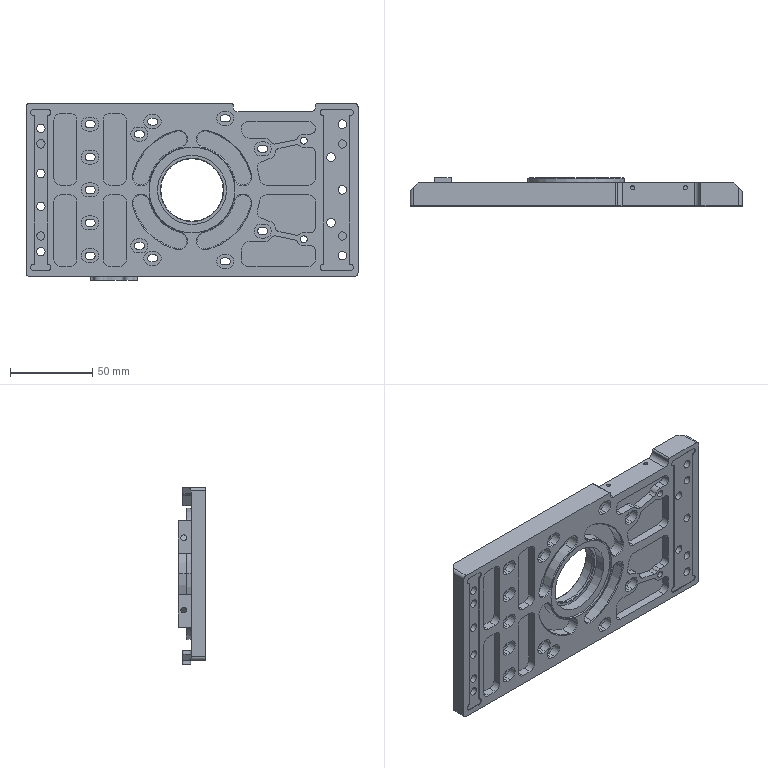NC program | Mastercam | posted with a generic post | part box 202 x 17 x 107.5 mm
Lines 3574 to 4550 of 36425:
(6 FEM |TOOL - 6|DIA. OFF. - 6|LEN. - 6|TOOL DIA. - 6.)
N7212 T6 M6
N7214 G0 G54 G90 X68.194 Y51.5 C0. B0. S6500 M3
N7216 G43 H6 Z100.
N7218 Z1.
N7220 G1 Z-.494 F600.
N7222 Y50.9 F3000.
N7224 G3 X68.494 Y50.6 I.3
N7226 G1 X71.9
N7228 Y51.5
N7230 G2 X72.969 Y54.261 I4.1
N7232 G3 X73.047 Y54.463 I-.222 J.202
N7234 X72.949 Y54.685 I-.3
N7236 G1 X72.506 Y55.089
N7238 X68.194 Y51.5
N7240 Z-.988 F600.
N7242 Y50.9 F3000.
N7244 G3 X68.494 Y50.6 I.3
N7246 G1 X71.9
N7248 Y51.5
N7250 G2 X72.969 Y54.261 I4.1
N7252 G3 X73.047 Y54.463 I-.222 J.202
N7254 X72.949 Y54.685 I-.3
N7256 G1 X72.506 Y55.089
N7258 X68.194 Y51.5
N7260 Z-1.482 F600.
N7262 Y50.9 F3000.
N7264 G3 X68.494 Y50.6 I.3
N7266 G1 X71.9
N7268 Y51.5
N7270 G2 X72.969 Y54.261 I4.1
N7272 G3 X73.047 Y54.463 I-.222 J.202
N7274 X72.949 Y54.685 I-.3
N7276 G1 X72.506 Y55.089
N7278 X68.194 Y51.5
N7280 Z-1.976 F600.
N7282 Y50.9 F3000.
N7284 G3 X68.494 Y50.6 I.3
N7286 G1 X71.9
N7288 Y51.5
N7290 G2 X72.969 Y54.261 I4.1
N7292 G3 X73.047 Y54.463 I-.222 J.202
N7294 X72.949 Y54.685 I-.3
N7296 G1 X72.506 Y55.089
N7298 X68.194 Y51.5
N7300 Z-2.471 F600.
N7302 Y50.9 F3000.
N7304 G3 X68.494 Y50.6 I.3
N7306 G1 X71.9
N7308 Y51.5
N7310 G2 X72.969 Y54.261 I4.1
N7312 G3 X73.047 Y54.463 I-.222 J.202
N7314 X72.949 Y54.685 I-.3
N7316 G1 X72.506 Y55.089
N7318 X68.194 Y51.5
N7320 Z-2.965 F600.
N7322 Y50.9 F3000.
N7324 G3 X68.494 Y50.6 I.3
N7326 G1 X71.9
N7328 Y51.5
N7330 G2 X72.969 Y54.261 I4.1
N7332 G3 X73.047 Y54.463 I-.222 J.202
N7334 X72.949 Y54.685 I-.3
N7336 G1 X72.506 Y55.089
N7338 X68.194 Y51.5
N7340 Z-3.459 F600.
N7342 Y50.9 F3000.
N7344 G3 X68.494 Y50.6 I.3
N7346 G1 X71.9
N7348 Y51.5
N7350 G2 X72.969 Y54.261 I4.1
N7352 G3 X73.047 Y54.463 I-.222 J.202
N7354 X72.949 Y54.685 I-.3
N7356 G1 X72.506 Y55.089
N7358 X68.194 Y51.5
N7360 Z-3.953 F600.
N7362 Y50.9 F3000.
N7364 G3 X68.494 Y50.6 I.3
N7366 G1 X71.9
N7368 Y51.5
N7370 G2 X72.969 Y54.261 I4.1
N7372 G3 X73.047 Y54.463 I-.222 J.202
N7374 X72.949 Y54.685 I-.3
N7376 G1 X72.506 Y55.089
N7378 X68.194 Y51.5
N7380 Z-4.447 F600.
N7382 Y50.9 F3000.
N7384 G3 X68.494 Y50.6 I.3
N7386 G1 X71.9
N7388 Y51.5
N7390 G2 X72.969 Y54.261 I4.1
N7392 G3 X73.047 Y54.463 I-.222 J.202
N7394 X72.949 Y54.685 I-.3
N7396 G1 X72.506 Y55.089
N7398 X68.194 Y51.5
N7400 Z-4.941 F600.
N7402 Y50.9 F3000.
N7404 G3 X68.494 Y50.6 I.3
N7406 G1 X71.9
N7408 Y51.5
N7410 G2 X72.969 Y54.261 I4.1
N7412 G3 X73.047 Y54.463 I-.222 J.202
N7414 X72.949 Y54.685 I-.3
N7416 G1 X72.506 Y55.089
N7418 X68.194 Y51.5
N7420 Z-5.435 F600.
N7422 Y50.9 F3000.
N7424 G3 X68.494 Y50.6 I.3
N7426 G1 X71.9
N7428 Y51.5
N7430 G2 X72.969 Y54.261 I4.1
N7432 G3 X73.047 Y54.463 I-.222 J.202
N7434 X72.949 Y54.685 I-.3
N7436 G1 X72.506 Y55.089
N7438 X68.194 Y51.5
N7440 Z-5.929 F600.
N7442 Y50.9 F3000.
N7444 G3 X68.494 Y50.6 I.3
N7446 G1 X71.9
N7448 Y51.5
N7450 G2 X72.969 Y54.261 I4.1
N7452 G3 X73.047 Y54.463 I-.222 J.202
N7454 X72.949 Y54.685 I-.3
N7456 G1 X72.506 Y55.089
N7458 X68.194 Y51.5
N7460 Z-6.424 F600.
N7462 Y50.9 F3000.
N7464 G3 X68.494 Y50.6 I.3
N7466 G1 X71.9
N7468 Y51.5
N7470 G2 X72.969 Y54.261 I4.1
N7472 G3 X73.047 Y54.463 I-.222 J.202
N7474 X72.949 Y54.685 I-.3
N7476 G1 X72.506 Y55.089
N7478 X68.194 Y51.5
N7480 Z-6.918 F600.
N7482 Y50.9 F3000.
N7484 G3 X68.494 Y50.6 I.3
N7486 G1 X71.9
N7488 Y51.5
N7490 G2 X72.969 Y54.261 I4.1
N7492 G3 X73.047 Y54.463 I-.222 J.202
N7494 X72.949 Y54.685 I-.3
N7496 G1 X72.506 Y55.089
N7498 X68.194 Y51.5
N7500 Z-7.412 F600.
N7502 Y50.9 F3000.
N7504 G3 X68.494 Y50.6 I.3
N7506 G1 X71.9
N7508 Y51.5
N7510 G2 X72.969 Y54.261 I4.1
N7512 G3 X73.047 Y54.463 I-.222 J.202
N7514 X72.949 Y54.685 I-.3
N7516 G1 X72.506 Y55.089
N7518 X68.194 Y51.5
N7520 Z-7.906 F600.
N7522 Y50.9 F3000.
N7524 G3 X68.494 Y50.6 I.3
N7526 G1 X71.9
N7528 Y51.5
N7530 G2 X72.969 Y54.261 I4.1
N7532 G3 X73.047 Y54.463 I-.222 J.202
N7534 X72.949 Y54.685 I-.3
N7536 G1 X72.506 Y55.089
N7538 X68.194 Y51.5
N7540 Z-8.4 F600.
N7542 Y50.9 F3000.
N7544 G3 X68.494 Y50.6 I.3
N7546 G1 X71.9
N7548 Y51.5
N7550 G2 X72.969 Y54.261 I4.1
N7552 G3 X73.047 Y54.463 I-.222 J.202
N7554 X72.949 Y54.685 I-.3
N7556 G1 X72.506 Y55.089
N7558 X68.194 Y51.5
N7560 Z-8.894 F600.
N7562 Y50.9 F3000.
N7564 G3 X68.494 Y50.6 I.3
N7566 G1 X71.9
N7568 Y51.5
N7570 G2 X72.969 Y54.261 I4.1
N7572 G3 X73.047 Y54.463 I-.222 J.202
N7574 X72.949 Y54.685 I-.3
N7576 G1 X72.506 Y55.089
N7578 X68.194 Y51.5
N7580 Z-9.388 F600.
N7582 Y50.9 F3000.
N7584 G3 X68.494 Y50.6 I.3
N7586 G1 X71.9
N7588 Y51.5
N7590 G2 X72.969 Y54.261 I4.1
N7592 G3 X73.047 Y54.463 I-.222 J.202
N7594 X72.949 Y54.685 I-.3
N7596 G1 X72.506 Y55.089
N7598 X68.194 Y51.5
N7600 Z-9.882 F600.
N7602 Y50.9 F3000.
N7604 G3 X68.494 Y50.6 I.3
N7606 G1 X71.9
N7608 Y51.5
N7610 G2 X72.969 Y54.261 I4.1
N7612 G3 X73.047 Y54.463 I-.222 J.202
N7614 X72.949 Y54.685 I-.3
N7616 G1 X72.506 Y55.089
N7618 X68.194 Y51.5
N7620 Z-10.376 F600.
N7622 Y50.9 F3000.
N7624 G3 X68.494 Y50.6 I.3
N7626 G1 X71.9
N7628 Y51.5
N7630 G2 X72.969 Y54.261 I4.1
N7632 G3 X73.047 Y54.463 I-.222 J.202
N7634 X72.949 Y54.685 I-.3
N7636 G1 X72.506 Y55.089
N7638 X68.194 Y51.5
N7640 Z-10.871 F600.
N7642 Y50.9 F3000.
N7644 G3 X68.494 Y50.6 I.3
N7646 G1 X71.9
N7648 Y51.5
N7650 G2 X72.969 Y54.261 I4.1
N7652 G3 X73.047 Y54.463 I-.222 J.202
N7654 X72.949 Y54.685 I-.3
N7656 G1 X72.506 Y55.089
N7658 X68.194 Y51.5
N7660 Z-11.365 F600.
N7662 Y50.9 F3000.
N7664 G3 X68.494 Y50.6 I.3
N7666 G1 X71.9
N7668 Y51.5
N7670 G2 X72.969 Y54.261 I4.1
N7672 G3 X73.047 Y54.463 I-.222 J.202
N7674 X72.949 Y54.685 I-.3
N7676 G1 X72.506 Y55.089
N7678 X68.194 Y51.5
N7680 Z-11.859 F600.
N7682 Y50.9 F3000.
N7684 G3 X68.494 Y50.6 I.3
N7686 G1 X71.9
N7688 Y51.5
N7690 G2 X72.969 Y54.261 I4.1
N7692 G3 X73.047 Y54.463 I-.222 J.202
N7694 X72.949 Y54.685 I-.3
N7696 G1 X72.506 Y55.089
N7698 X68.194 Y51.5
N7700 Z-12.353 F600.
N7702 Y50.9 F3000.
N7704 G3 X68.494 Y50.6 I.3
N7706 G1 X71.9
N7708 Y51.5
N7710 G2 X72.969 Y54.261 I4.1
N7712 G3 X73.047 Y54.463 I-.222 J.202
N7714 X72.949 Y54.685 I-.3
N7716 G1 X72.506 Y55.089
N7718 X68.194 Y51.5
N7720 Z-12.847 F600.
N7722 Y50.9 F3000.
N7724 G3 X68.494 Y50.6 I.3
N7726 G1 X71.9
N7728 Y51.5
N7730 G2 X72.969 Y54.261 I4.1
N7732 G3 X73.047 Y54.463 I-.222 J.202
N7734 X72.949 Y54.685 I-.3
N7736 G1 X72.506 Y55.089
N7738 X68.194 Y51.5
N7740 Z-13.341 F600.
N7742 Y50.9 F3000.
N7744 G3 X68.494 Y50.6 I.3
N7746 G1 X71.9
N7748 Y51.5
N7750 G2 X72.969 Y54.261 I4.1
N7752 G3 X73.047 Y54.463 I-.222 J.202
N7754 X72.949 Y54.685 I-.3
N7756 G1 X72.506 Y55.089
N7758 X68.194 Y51.5
N7760 Z-13.835 F600.
N7762 Y50.9 F3000.
N7764 G3 X68.494 Y50.6 I.3
N7766 G1 X71.9
N7768 Y51.5
N7770 G2 X72.969 Y54.261 I4.1
N7772 G3 X73.047 Y54.463 I-.222 J.202
N7774 X72.949 Y54.685 I-.3
N7776 G1 X72.506 Y55.089
N7778 X68.194 Y51.5
N7780 Z-14.329 F600.
N7782 Y50.9 F3000.
N7784 G3 X68.494 Y50.6 I.3
N7786 G1 X71.9
N7788 Y51.5
N7790 G2 X72.969 Y54.261 I4.1
N7792 G3 X73.047 Y54.463 I-.222 J.202
N7794 X72.949 Y54.685 I-.3
N7796 G1 X72.506 Y55.089
N7798 X68.194 Y51.5
N7800 Z-14.824 F600.
N7802 Y50.9 F3000.
N7804 G3 X68.494 Y50.6 I.3
N7806 G1 X71.9
N7808 Y51.5
N7810 G2 X72.969 Y54.261 I4.1
N7812 G3 X73.047 Y54.463 I-.222 J.202
N7814 X72.949 Y54.685 I-.3
N7816 G1 X72.506 Y55.089
N7818 X68.194 Y51.5
N7820 Z-15.318 F600.
N7822 Y50.9 F3000.
N7824 G3 X68.494 Y50.6 I.3
N7826 G1 X71.9
N7828 Y51.5
N7830 G2 X72.969 Y54.261 I4.1
N7832 G3 X73.047 Y54.463 I-.222 J.202
N7834 X72.949 Y54.685 I-.3
N7836 G1 X72.506 Y55.089
N7838 X68.194 Y51.5
N7840 Z-15.812 F600.
N7842 Y50.9 F3000.
N7844 G3 X68.494 Y50.6 I.3
N7846 G1 X71.9
N7848 Y51.5
N7850 G2 X72.969 Y54.261 I4.1
N7852 G3 X73.047 Y54.463 I-.222 J.202
N7854 X72.949 Y54.685 I-.3
N7856 G1 X72.506 Y55.089
N7858 X68.194 Y51.5
N7860 Z-16.306 F600.
N7862 Y50.9 F3000.
N7864 G3 X68.494 Y50.6 I.3
N7866 G1 X71.9
N7868 Y51.5
N7870 G2 X72.969 Y54.261 I4.1
N7872 G3 X73.047 Y54.463 I-.222 J.202
N7874 X72.949 Y54.685 I-.3
N7876 G1 X72.506 Y55.089
N7878 X68.194 Y51.5
N7880 Z-16.8 F600.
N7882 Y50.9 F3000.
N7884 G3 X68.494 Y50.6 I.3
N7886 G1 X71.9
N7888 Y51.5
N7890 G2 X72.969 Y54.261 I4.1
N7892 G3 X73.047 Y54.463 I-.222 J.202
N7894 X72.949 Y54.685 I-.3
N7896 G1 X72.506 Y55.089
N7898 Z-15.8 F1200.
N7900 G0 Z100.
N7902 X27.48 Y55.103
N7904 Z1.
N7906 G1 Z-.494 F600.
N7908 X27.038 Y54.697 F3000.
N7910 G3 X26.941 Y54.476 I.203 J-.221
N7912 X27.02 Y54.273 I.3
N7914 G2 X28.1 Y51.5 I-3.02 J-2.773
N7916 G1 Y50.6
N7918 X31.52
N7920 G3 X31.82 Y50.9 J.3
N7922 G1 Y51.5
N7924 X27.48 Y55.103
N7926 Z-.988 F600.
N7928 X27.038 Y54.697 F3000.
N7930 G3 X26.941 Y54.476 I.203 J-.221
N7932 X27.02 Y54.273 I.3
N7934 G2 X28.1 Y51.5 I-3.02 J-2.773
N7936 G1 Y50.6
N7938 X31.52
N7940 G3 X31.82 Y50.9 J.3
N7942 G1 Y51.5
N7944 X27.48 Y55.103
N7946 Z-1.482 F600.
N7948 X27.038 Y54.697 F3000.
N7950 G3 X26.941 Y54.476 I.203 J-.221
N7952 X27.02 Y54.273 I.3
N7954 G2 X28.1 Y51.5 I-3.02 J-2.773
N7956 G1 Y50.6
N7958 X31.52
N7960 G3 X31.82 Y50.9 J.3
N7962 G1 Y51.5
N7964 X27.48 Y55.103
N7966 Z-1.976 F600.
N7968 X27.038 Y54.697 F3000.
N7970 G3 X26.941 Y54.476 I.203 J-.221
N7972 X27.02 Y54.273 I.3
N7974 G2 X28.1 Y51.5 I-3.02 J-2.773
N7976 G1 Y50.6
N7978 X31.52
N7980 G3 X31.82 Y50.9 J.3
N7982 G1 Y51.5
N7984 X27.48 Y55.103
N7986 Z-2.471 F600.
N7988 X27.038 Y54.697 F3000.
N7990 G3 X26.941 Y54.476 I.203 J-.221
N7992 X27.02 Y54.273 I.3
N7994 G2 X28.1 Y51.5 I-3.02 J-2.773
N7996 G1 Y50.6
N7998 X31.52
N8000 G3 X31.82 Y50.9 J.3
N8002 G1 Y51.5
N8004 X27.48 Y55.103
N8006 Z-2.965 F600.
N8008 X27.038 Y54.697 F3000.
N8010 G3 X26.941 Y54.476 I.203 J-.221
N8012 X27.02 Y54.273 I.3
N8014 G2 X28.1 Y51.5 I-3.02 J-2.773
N8016 G1 Y50.6
N8018 X31.52
N8020 G3 X31.82 Y50.9 J.3
N8022 G1 Y51.5
N8024 X27.48 Y55.103
N8026 Z-3.459 F600.
N8028 X27.038 Y54.697 F3000.
N8030 G3 X26.941 Y54.476 I.203 J-.221
N8032 X27.02 Y54.273 I.3
N8034 G2 X28.1 Y51.5 I-3.02 J-2.773
N8036 G1 Y50.6
N8038 X31.52
N8040 G3 X31.82 Y50.9 J.3
N8042 G1 Y51.5
N8044 X27.48 Y55.103
N8046 Z-3.953 F600.
N8048 X27.038 Y54.697 F3000.
N8050 G3 X26.941 Y54.476 I.203 J-.221
N8052 X27.02 Y54.273 I.3
N8054 G2 X28.1 Y51.5 I-3.02 J-2.773
N8056 G1 Y50.6
N8058 X31.52
N8060 G3 X31.82 Y50.9 J.3
N8062 G1 Y51.5
N8064 X27.48 Y55.103
N8066 Z-4.447 F600.
N8068 X27.038 Y54.697 F3000.
N8070 G3 X26.941 Y54.476 I.203 J-.221
N8072 X27.02 Y54.273 I.3
N8074 G2 X28.1 Y51.5 I-3.02 J-2.773
N8076 G1 Y50.6
N8078 X31.52
N8080 G3 X31.82 Y50.9 J.3
N8082 G1 Y51.5
N8084 X27.48 Y55.103
N8086 Z-4.941 F600.
N8088 X27.038 Y54.697 F3000.
N8090 G3 X26.941 Y54.476 I.203 J-.221
N8092 X27.02 Y54.273 I.3
N8094 G2 X28.1 Y51.5 I-3.02 J-2.773
N8096 G1 Y50.6
N8098 X31.52
N8100 G3 X31.82 Y50.9 J.3
N8102 G1 Y51.5
N8104 X27.48 Y55.103
N8106 Z-5.435 F600.
N8108 X27.038 Y54.697 F3000.
N8110 G3 X26.941 Y54.476 I.203 J-.221
N8112 X27.02 Y54.273 I.3
N8114 G2 X28.1 Y51.5 I-3.02 J-2.773
N8116 G1 Y50.6
N8118 X31.52
N8120 G3 X31.82 Y50.9 J.3
N8122 G1 Y51.5
N8124 X27.48 Y55.103
N8126 Z-5.929 F600.
N8128 X27.038 Y54.697 F3000.
N8130 G3 X26.941 Y54.476 I.203 J-.221
N8132 X27.02 Y54.273 I.3
N8134 G2 X28.1 Y51.5 I-3.02 J-2.773
N8136 G1 Y50.6
N8138 X31.52
N8140 G3 X31.82 Y50.9 J.3
N8142 G1 Y51.5
N8144 X27.48 Y55.103
N8146 Z-6.424 F600.
N8148 X27.038 Y54.697 F3000.
N8150 G3 X26.941 Y54.476 I.203 J-.221
N8152 X27.02 Y54.273 I.3
N8154 G2 X28.1 Y51.5 I-3.02 J-2.773
N8156 G1 Y50.6
N8158 X31.52
N8160 G3 X31.82 Y50.9 J.3
N8162 G1 Y51.5
N8164 X27.48 Y55.103
N8166 Z-6.918 F600.
N8168 X27.038 Y54.697 F3000.
N8170 G3 X26.941 Y54.476 I.203 J-.221
N8172 X27.02 Y54.273 I.3
N8174 G2 X28.1 Y51.5 I-3.02 J-2.773
N8176 G1 Y50.6
N8178 X31.52
N8180 G3 X31.82 Y50.9 J.3
N8182 G1 Y51.5
N8184 X27.48 Y55.103
N8186 Z-7.412 F600.
N8188 X27.038 Y54.697 F3000.
N8190 G3 X26.941 Y54.476 I.203 J-.221
N8192 X27.02 Y54.273 I.3
N8194 G2 X28.1 Y51.5 I-3.02 J-2.773
N8196 G1 Y50.6
N8198 X31.52
N8200 G3 X31.82 Y50.9 J.3
N8202 G1 Y51.5
N8204 X27.48 Y55.103
N8206 Z-7.906 F600.
N8208 X27.038 Y54.697 F3000.
N8210 G3 X26.941 Y54.476 I.203 J-.221
N8212 X27.02 Y54.273 I.3
N8214 G2 X28.1 Y51.5 I-3.02 J-2.773
N8216 G1 Y50.6
N8218 X31.52
N8220 G3 X31.82 Y50.9 J.3
N8222 G1 Y51.5
N8224 X27.48 Y55.103
N8226 Z-8.4 F600.
N8228 X27.038 Y54.697 F3000.
N8230 G3 X26.941 Y54.476 I.203 J-.221
N8232 X27.02 Y54.273 I.3
N8234 G2 X28.1 Y51.5 I-3.02 J-2.773
N8236 G1 Y50.6
N8238 X31.52
N8240 G3 X31.82 Y50.9 J.3
N8242 G1 Y51.5
N8244 X27.48 Y55.103
N8246 Z-8.894 F600.
N8248 X27.038 Y54.697 F3000.
N8250 G3 X26.941 Y54.476 I.203 J-.221
N8252 X27.02 Y54.273 I.3
N8254 G2 X28.1 Y51.5 I-3.02 J-2.773
N8256 G1 Y50.6
N8258 X31.52
N8260 G3 X31.82 Y50.9 J.3
N8262 G1 Y51.5
N8264 X27.48 Y55.103
N8266 Z-9.388 F600.
N8268 X27.038 Y54.697 F3000.
N8270 G3 X26.941 Y54.476 I.203 J-.221
N8272 X27.02 Y54.273 I.3
N8274 G2 X28.1 Y51.5 I-3.02 J-2.773
N8276 G1 Y50.6
N8278 X31.52
N8280 G3 X31.82 Y50.9 J.3
N8282 G1 Y51.5
N8284 X27.48 Y55.103
N8286 Z-9.882 F600.
N8288 X27.038 Y54.697 F3000.
N8290 G3 X26.941 Y54.476 I.203 J-.221
N8292 X27.02 Y54.273 I.3
N8294 G2 X28.1 Y51.5 I-3.02 J-2.773
N8296 G1 Y50.6
N8298 X31.52
N8300 G3 X31.82 Y50.9 J.3
N8302 G1 Y51.5
N8304 X27.48 Y55.103
N8306 Z-10.376 F600.
N8308 X27.038 Y54.697 F3000.
N8310 G3 X26.941 Y54.476 I.203 J-.221
N8312 X27.02 Y54.273 I.3
N8314 G2 X28.1 Y51.5 I-3.02 J-2.773
N8316 G1 Y50.6
N8318 X31.52
N8320 G3 X31.82 Y50.9 J.3
N8322 G1 Y51.5
N8324 X27.48 Y55.103
N8326 Z-10.871 F600.
N8328 X27.038 Y54.697 F3000.
N8330 G3 X26.941 Y54.476 I.203 J-.221
N8332 X27.02 Y54.273 I.3
N8334 G2 X28.1 Y51.5 I-3.02 J-2.773
N8336 G1 Y50.6
N8338 X31.52
N8340 G3 X31.82 Y50.9 J.3
N8342 G1 Y51.5
N8344 X27.48 Y55.103
N8346 Z-11.365 F600.
N8348 X27.038 Y54.697 F3000.
N8350 G3 X26.941 Y54.476 I.203 J-.221
N8352 X27.02 Y54.273 I.3
N8354 G2 X28.1 Y51.5 I-3.02 J-2.773
N8356 G1 Y50.6
N8358 X31.52
N8360 G3 X31.82 Y50.9 J.3
N8362 G1 Y51.5
N8364 X27.48 Y55.103
N8366 Z-11.859 F600.
N8368 X27.038 Y54.697 F3000.
N8370 G3 X26.941 Y54.476 I.203 J-.221
N8372 X27.02 Y54.273 I.3
N8374 G2 X28.1 Y51.5 I-3.02 J-2.773
N8376 G1 Y50.6
N8378 X31.52
N8380 G3 X31.82 Y50.9 J.3
N8382 G1 Y51.5
N8384 X27.48 Y55.103
N8386 Z-12.353 F600.
N8388 X27.038 Y54.697 F3000.
N8390 G3 X26.941 Y54.476 I.203 J-.221
N8392 X27.02 Y54.273 I.3
N8394 G2 X28.1 Y51.5 I-3.02 J-2.773
N8396 G1 Y50.6
N8398 X31.52
N8400 G3 X31.82 Y50.9 J.3
N8402 G1 Y51.5
N8404 X27.48 Y55.103
N8406 Z-12.847 F600.
N8408 X27.038 Y54.697 F3000.
N8410 G3 X26.941 Y54.476 I.203 J-.221
N8412 X27.02 Y54.273 I.3
N8414 G2 X28.1 Y51.5 I-3.02 J-2.773
N8416 G1 Y50.6
N8418 X31.52
N8420 G3 X31.82 Y50.9 J.3
N8422 G1 Y51.5
N8424 X27.48 Y55.103
N8426 Z-13.341 F600.
N8428 X27.038 Y54.697 F3000.
N8430 G3 X26.941 Y54.476 I.203 J-.221
N8432 X27.02 Y54.273 I.3
N8434 G2 X28.1 Y51.5 I-3.02 J-2.773
N8436 G1 Y50.6
N8438 X31.52
N8440 G3 X31.82 Y50.9 J.3
N8442 G1 Y51.5
N8444 X27.48 Y55.103
N8446 Z-13.835 F600.
N8448 X27.038 Y54.697 F3000.
N8450 G3 X26.941 Y54.476 I.203 J-.221
N8452 X27.02 Y54.273 I.3
N8454 G2 X28.1 Y51.5 I-3.02 J-2.773
N8456 G1 Y50.6
N8458 X31.52
N8460 G3 X31.82 Y50.9 J.3
N8462 G1 Y51.5
N8464 X27.48 Y55.103
N8466 Z-14.329 F600.
N8468 X27.038 Y54.697 F3000.
N8470 G3 X26.941 Y54.476 I.203 J-.221
N8472 X27.02 Y54.273 I.3
N8474 G2 X28.1 Y51.5 I-3.02 J-2.773
N8476 G1 Y50.6
N8478 X31.52
N8480 G3 X31.82 Y50.9 J.3
N8482 G1 Y51.5
N8484 X27.48 Y55.103
N8486 Z-14.824 F600.
N8488 X27.038 Y54.697 F3000.
N8490 G3 X26.941 Y54.476 I.203 J-.221
N8492 X27.02 Y54.273 I.3
N8494 G2 X28.1 Y51.5 I-3.02 J-2.773
N8496 G1 Y50.6
N8498 X31.52
N8500 G3 X31.82 Y50.9 J.3
N8502 G1 Y51.5
N8504 X27.48 Y55.103
N8506 Z-15.318 F600.
N8508 X27.038 Y54.697 F3000.
N8510 G3 X26.941 Y54.476 I.203 J-.221
N8512 X27.02 Y54.273 I.3
N8514 G2 X28.1 Y51.5 I-3.02 J-2.773
N8516 G1 Y50.6
N8518 X31.52
N8520 G3 X31.82 Y50.9 J.3
N8522 G1 Y51.5
N8524 X27.48 Y55.103
N8526 Z-15.812 F600.
N8528 X27.038 Y54.697 F3000.
N8530 G3 X26.941 Y54.476 I.203 J-.221
N8532 X27.02 Y54.273 I.3
N8534 G2 X28.1 Y51.5 I-3.02 J-2.773
N8536 G1 Y50.6
N8538 X31.52
N8540 G3 X31.82 Y50.9 J.3
N8542 G1 Y51.5
N8544 X27.48 Y55.103
N8546 Z-16.306 F600.
N8548 X27.038 Y54.697 F3000.
N8550 G3 X26.941 Y54.476 I.203 J-.221
N8552 X27.02 Y54.273 I.3
N8554 G2 X28.1 Y51.5 I-3.02 J-2.773
N8556 G1 Y50.6
N8558 X31.52
N8560 G3 X31.82 Y50.9 J.3
N8562 G1 Y51.5
N8564 X27.48 Y55.103
N8566 Z-16.8 F600.
N8568 X27.038 Y54.697 F3000.
N8570 G3 X26.941 Y54.476 I.203 J-.221
N8572 X27.02 Y54.273 I.3
N8574 G2 X28.1 Y51.5 I-3.02 J-2.773
N8576 G1 Y50.6
N8578 X31.52
N8580 G3 X31.82 Y50.9 J.3
N8582 G1 Y51.5
N8584 Z-15.8 F1200.
N8586 G0 Z100.
N8588 X68.099 Y51.4
N8590 Z1.
N8592 G1 Z-4.2 F600.
N8594 Y50.8 F1000.
N8596 G3 X68.399 Y50.5 I.3
N8598 G1 X72.
N8600 Y51.5
N8602 G2 X73.16 Y54.316 I4.
N8604 G3 X73.248 Y54.528 I-.213 J.212
N8606 X73.158 Y54.741 I-.301
N8608 G1 X72.732 Y55.163
N8610 X68.099 Y51.4
N8612 Z-8.4 F600.
N8614 Y50.8 F1000.
N8616 G3 X68.399 Y50.5 I.3
N8618 G1 X72.
N8620 Y51.5
N8622 G2 X73.16 Y54.316 I4.
N8624 G3 X73.248 Y54.528 I-.213 J.212
N8626 X73.158 Y54.741 I-.301
N8628 G1 X72.732 Y55.163
N8630 X68.099 Y51.4
N8632 Z-12.6 F600.
N8634 Y50.8 F1000.
N8636 G3 X68.399 Y50.5 I.3
N8638 G1 X72.
N8640 Y51.5
N8642 G2 X73.16 Y54.316 I4.
N8644 G3 X73.248 Y54.528 I-.213 J.212
N8646 X73.158 Y54.741 I-.301
N8648 G1 X72.732 Y55.163
N8650 X68.099 Y51.4
N8652 Z-16.8 F600.
N8654 Y50.8 F1000.
N8656 G3 X68.399 Y50.5 I.3
N8658 G1 X72.
N8660 Y51.5
N8662 G2 X73.16 Y54.316 I4.
N8664 G3 X73.248 Y54.528 I-.213 J.212
N8666 X73.158 Y54.741 I-.301
N8668 G1 X72.732 Y55.163
N8670 Z-15.8 F1200.
N8672 G0 Z100.
N8674 X27.212 Y55.213
N8676 Z1.
N8678 G1 Z-4.2 F600.
N8680 X26.792 Y54.784 F1000.
N8682 G3 X26.706 Y54.574 I.215 J-.21
N8684 X26.797 Y54.36 I.301
N8686 G2 X28. Y51.5 I-2.797 J-2.86
N8688 G1 Y50.5
N8690 X31.602
N8692 G3 X31.902 Y50.8 J.3
N8694 G1 Y51.4
N8696 X27.212 Y55.213
N8698 Z-8.4 F600.
N8700 X26.792 Y54.784 F1000.
N8702 G3 X26.706 Y54.574 I.215 J-.21
N8704 X26.797 Y54.36 I.301
N8706 G2 X28. Y51.5 I-2.797 J-2.86
N8708 G1 Y50.5
N8710 X31.602
N8712 G3 X31.902 Y50.8 J.3
N8714 G1 Y51.4
N8716 X27.212 Y55.213
N8718 Z-12.6 F600.
N8720 X26.792 Y54.784 F1000.
N8722 G3 X26.706 Y54.574 I.215 J-.21
N8724 X26.797 Y54.36 I.301
N8726 G2 X28. Y51.5 I-2.797 J-2.86
N8728 G1 Y50.5
N8730 X31.602
N8732 G3 X31.902 Y50.8 J.3
N8734 G1 Y51.4
N8736 X27.212 Y55.213
N8738 Z-16.8 F600.
N8740 X26.792 Y54.784 F1000.
N8742 G3 X26.706 Y54.574 I.215 J-.21
N8744 X26.797 Y54.36 I.301
N8746 G2 X28. Y51.5 I-2.797 J-2.86
N8748 G1 Y50.5
N8750 X31.602
N8752 G3 X31.902 Y50.8 J.3
N8754 G1 Y51.4
N8756 Z-15.8 F1200.
N8758 G0 Z100.
N8760 S10000 M3
N8762 X61.633 Y13.206
N8764 Z30.
N8766 Z1.
N8768 G1 Z.3 F600.
N8770 X64.794 Z.273 F4000.
N8772 Y16.169 Z.255
N8774 G2 X62.798 Y16.782 Z.244 I3.223 J14.047
N8776 G1 X62.508 Y16.899 Z.241
N8778 X58.936 Y16.154 Z.21
N8780 X56.719 Y13.206 Z.187
N8782 X64.794 Z.132
N8784 Y16.169 Z.114
N8786 G2 X62.793 Y16.784 Z.103 I3.223 J14.047
N8788 G1 X62.508 Y16.899 Z.1
N8790 X58.936 Y16.154 Z.069
N8792 X56.719 Y13.206 Z.046
N8794 X64.794 Z-.009
N8796 Y16.169 Z-.028
N8798 G2 X62.813 Y16.777 Z-.038 I3.223 J14.047
N8800 G1 X62.508 Y16.899 Z-.041
N8802 X58.936 Y16.154 Z-.072
N8804 X56.719 Y13.206 Z-.095
N8806 X64.794 Z-.15
N8808 Y16.169 Z-.168
N8810 G2 X62.736 Y16.807 Z-.179 I3.223 J14.047
N8812 G1 X62.508 Y16.899 Z-.182
N8814 X58.936 Y16.154 Z-.212
N8816 X56.719 Y13.206 Z-.236
N8818 X64.794 Z-.292
N8820 Y16.169 Z-.313
N8822 G2 X63.133 Y16.657 Z-.321 I3.223 J14.047
N8824 X62.508 Y16.899 Z-.326 I4.884 J13.559
N8826 G1 X59.848 Y16.344 Z-.349
N8828 X58.936 Y16.154 Z-.357
N8830 X57.408 Y14.122 Z-.377
N8832 X56.719 Y13.206
N8834 X64.794
N8836 Y16.169
N8838 G2 X62.508 Y16.899 I3.223 J14.047
N8840 G1 X58.936 Y16.154
N8842 X57.408 Y14.122
N8844 G2 X56.914 Y13.876 I-.494 J.372
N8846 X56.679 Y13.922 J.618
N8848 G1 X54.359 Y14.873
N8850 G3 X54.125 Y14.919 I-.234 J-.572
N8852 X53.702 Y14.753 J-.618
N8854 G2 X53.61 Y14.667 I-9.402 J10.035
N8856 X47.356 Y11.576 I-13.987 J20.422
N8858 G1 X47.715 Y10.007
N8860 X67.993
N8862 Y18.995
N8864 G2 X62.91 Y20.25 I.632 J13.479
N8866 G1 X56.759 Y18.969
N8868 G2 X53.702 Y14.753 I-12.459 J5.819
N8870 X53.278 Y14.585 I-.424 J.451
N8872 X52.915 Y14.704 J.619
N8874 G1 X50.227 Y16.658
N8876 G3 X49.863 Y16.776 I-.364 J-.501
N8878 X49.597 Y16.716 J-.619
N8880 G2 X49.487 Y16.664 I-3.262 J6.849
N8882 G1 X43.821 Y14.361
N8884 X43.287 Y14.121
N8886 G3 X42.868 Y13.356 I.488 J-.765
N8888 X42.869 Y13.327 I.907
N8890 G1 X42.973 Y12.82
N8892 G2 X43.898 Y9.175 I-42.639 J-12.752
N8894 G1 X44.359 Y6.745
N8896 G3 X45.035 Y6.129 I.864 J.269
N8898 G1 X45.44 Y6.1
N8900 X70.936 Y6.104
N8902 X70.961
N8904 G3 X71.676 Y6.424 J.958
N8906 G1 X71.807 Y6.627
N8908 X71.852 Y6.745
N8910 X71.9 Y7.15
N8912 X71.898 Y22.897
N8914 X68.103 Y22.9
N8916 G2 X66.889 Y22.99 I.498 J14.905
N8918 X63.64 Y24.386 I1.222 J7.323
N8920 G1 X53.717 Y22.326
N8922 X53.629 Y22.301
N8924 G2 X52.994 Y20.11 I-7.888 J1.098
N8926 X51.106 Y17.666 I-6.654 J3.191
N8928 X49.597 Y16.716 I-4.771 J5.899
N8930 G0 Z30.
N8932 X61.633 Y13.206
N8934 Z.623
N8936 G1 Z-.077 F600.
N8938 X64.794 Z-.104 F4000.
N8940 Y16.169 Z-.122
N8942 G2 X62.798 Y16.782 Z-.133 I3.223 J14.047
N8944 G1 X62.508 Y16.899 Z-.136
N8946 X58.936 Y16.154 Z-.167
N8948 X56.719 Y13.206 Z-.189
N8950 X64.794 Z-.245
N8952 Y16.169 Z-.263
N8954 G2 X62.793 Y16.784 Z-.274 I3.223 J14.047
N8956 G1 X62.508 Y16.899 Z-.277
N8958 X58.936 Y16.154 Z-.308
N8960 X56.719 Y13.206 Z-.33
N8962 X64.794 Z-.386
N8964 Y16.169 Z-.405
N8966 G2 X62.813 Y16.777 Z-.415 I3.223 J14.047
N8968 G1 X62.508 Y16.899 Z-.418
N8970 X58.936 Y16.154 Z-.449
N8972 X56.719 Y13.206 Z-.472
N8974 X64.794 Z-.527
N8976 Y16.169 Z-.545
N8978 G2 X62.736 Y16.807 Z-.556 I3.223 J14.047
N8980 G1 X62.508 Y16.899 Z-.559
N8982 X58.936 Y16.154 Z-.589
N8984 X56.719 Y13.206 Z-.613
N8986 X64.794 Z-.669
N8988 Y16.169 Z-.689
N8990 G2 X63.133 Y16.657 Z-.697 I3.223 J14.047
N8992 X62.508 Y16.899 Z-.703 I4.884 J13.559
N8994 G1 X59.848 Y16.344 Z-.726
N8996 X58.936 Y16.154 Z-.734
N8998 X57.408 Y14.122 Z-.754
N9000 X56.719 Y13.206
N9002 X64.794
N9004 Y16.169
N9006 G2 X62.508 Y16.899 I3.223 J14.047
N9008 G1 X58.936 Y16.154
N9010 X57.408 Y14.122
N9012 G2 X56.914 Y13.876 I-.494 J.372
N9014 X56.679 Y13.922 J.618
N9016 G1 X54.359 Y14.873
N9018 G3 X54.125 Y14.919 I-.234 J-.572
N9020 X53.702 Y14.753 J-.618
N9022 G2 X53.61 Y14.667 I-9.402 J10.035
N9024 X47.356 Y11.576 I-13.987 J20.422
N9026 G1 X47.715 Y10.007
N9028 X67.993
N9030 Y18.995
N9032 G2 X62.91 Y20.25 I.632 J13.479
N9034 G1 X56.759 Y18.969
N9036 G2 X53.702 Y14.753 I-12.459 J5.819
N9038 X53.278 Y14.585 I-.424 J.451
N9040 X52.915 Y14.704 J.619
N9042 G1 X50.227 Y16.658
N9044 G3 X49.863 Y16.776 I-.364 J-.501
N9046 X49.597 Y16.716 J-.619
N9048 G2 X49.487 Y16.664 I-3.262 J6.849
N9050 G1 X43.821 Y14.361
N9052 X43.287 Y14.121
N9054 G3 X42.868 Y13.356 I.488 J-.765
N9056 X42.869 Y13.327 I.907
N9058 G1 X42.973 Y12.82
N9060 G2 X43.898 Y9.175 I-42.639 J-12.752
N9062 G1 X44.359 Y6.745
N9064 G3 X45.035 Y6.129 I.864 J.269
N9066 G1 X45.44 Y6.1
N9068 X70.936 Y6.104
N9070 X70.961
N9072 G3 X71.676 Y6.424 J.958
N9074 G1 X71.807 Y6.627
N9076 X71.852 Y6.745
N9078 X71.9 Y7.15
N9080 X71.898 Y22.897
N9082 X68.103 Y22.9
N9084 G2 X66.889 Y22.99 I.498 J14.905
N9086 X63.64 Y24.386 I1.222 J7.323
N9088 G1 X53.717 Y22.326
N9090 X53.629 Y22.301
N9092 G2 X52.994 Y20.11 I-7.888 J1.098
N9094 X51.106 Y17.666 I-6.654 J3.191
N9096 X49.597 Y16.716 I-4.771 J5.899
N9098 G0 Z30.
N9100 X61.633 Y13.206
N9102 Z.246
N9104 G1 Z-.454 F600.
N9106 X64.794 Z-.481 F4000.
N9108 Y16.169 Z-.499
N9110 G2 X62.798 Y16.782 Z-.51 I3.223 J14.047
N9112 G1 X62.508 Y16.899 Z-.513
N9114 X58.936 Y16.154 Z-.544
N9116 X56.719 Y13.206 Z-.566
N9118 X64.794 Z-.622
N9120 Y16.169 Z-.64
N9122 G2 X62.793 Y16.784 Z-.651 I3.223 J14.047
N9124 G1 X62.508 Y16.899 Z-.654
N9126 X58.936 Y16.154 Z-.685
N9128 X56.719 Y13.206 Z-.707
N9130 X64.794 Z-.763
N9132 Y16.169 Z-.781
N9134 G2 X62.813 Y16.777 Z-.792 I3.223 J14.047
N9136 G1 X62.508 Y16.899 Z-.795
N9138 X58.936 Y16.154 Z-.826
N9140 X56.719 Y13.206 Z-.848
N9142 X64.794 Z-.904
N9144 Y16.169 Z-.922
N9146 G2 X62.736 Y16.807 Z-.933 I3.223 J14.047
N9148 G1 X62.508 Y16.899 Z-.935
N9150 X58.936 Y16.154 Z-.966
N9152 X56.719 Y13.206 Z-.99
N9154 X64.794 Z-1.046
N9156 Y16.169 Z-1.066
N9158 G2 X63.133 Y16.657 Z-1.074 I3.223 J14.047
N9160 X62.508 Y16.899 Z-1.08 I4.884 J13.559
N9162 G1 X59.848 Y16.344 Z-1.103